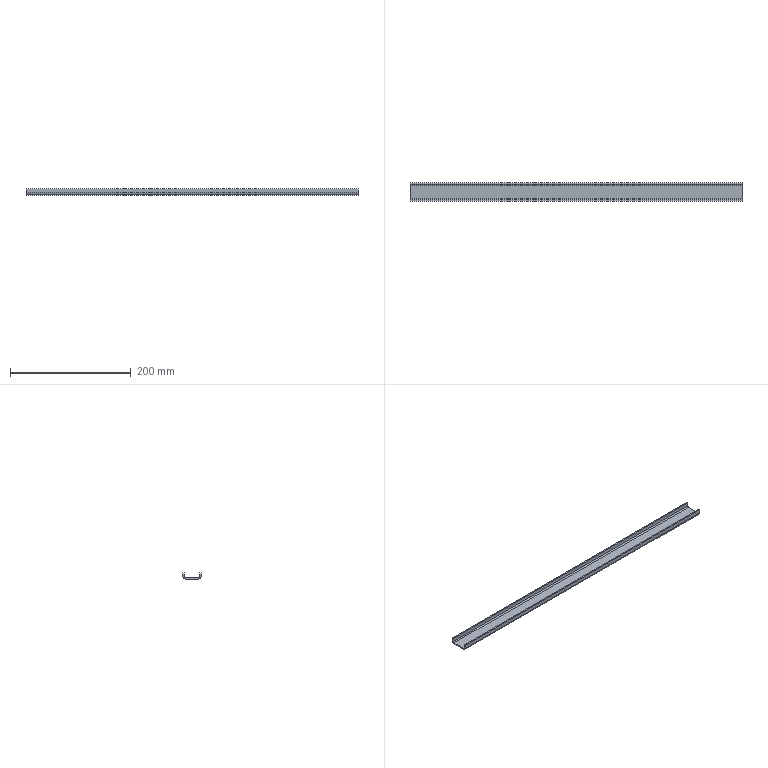Part | NX | features solid 2 | 1 solid | 14 faces | box 550 x 30 x 10 mm | volume 47767 mm3 | plane 10 | cylinder 4 | commonest cylinder face diameters 4 x2 8 x2
STEP:
#1=CARTESIAN_POINT('',(1955.,-1075.,1448.8));
#2=VERTEX_POINT('',#1);
#3=CARTESIAN_POINT('',(1955.,-1075.,1454.8));
#4=VERTEX_POINT('',#3);
#5=CARTESIAN_POINT('',(1955.,-1075.,1444.8));
#6=DIRECTION('',(0.,0.,1.));
#7=VECTOR('',#6,1000.);
#8=LINE('',#5,#7);
#9=EDGE_CURVE('',#2,#4,#8,.T.);
#10=ORIENTED_EDGE('',*,*,#9,.T.);
#11=CARTESIAN_POINT('',(1405.,-1075.,1454.8));
#12=VERTEX_POINT('',#11);
#13=CARTESIAN_POINT('',(1405.,-1075.,1454.8));
#14=DIRECTION('',(1.,0.,0.));
#15=VECTOR('',#14,1000.);
#16=LINE('',#13,#15);
#17=EDGE_CURVE('',#12,#4,#16,.T.);
#18=ORIENTED_EDGE('',*,*,#17,.F.);
#19=CARTESIAN_POINT('',(1405.,-1075.,1448.8));
#20=VERTEX_POINT('',#19);
#21=CARTESIAN_POINT('',(1405.,-1075.,1444.8));
#22=DIRECTION('',(0.,0.,1.));
#23=VECTOR('',#22,1000.);
#24=LINE('',#21,#23);
#25=EDGE_CURVE('',#20,#12,#24,.T.);
#26=ORIENTED_EDGE('',*,*,#25,.F.);
#27=CARTESIAN_POINT('',(1405.,-1075.,1448.8));
#28=DIRECTION('',(1.,0.,0.));
#29=VECTOR('',#28,1000.);
#30=LINE('',#27,#29);
#31=EDGE_CURVE('',#20,#2,#30,.T.);
#32=ORIENTED_EDGE('',*,*,#31,.T.);
#33=EDGE_LOOP('',(#10,#18,#26,#32));
#34=FACE_BOUND('',#33,.T.);
#35=CARTESIAN_POINT('',(1405.,-1075.,1444.8));
#36=DIRECTION('',(0.,1.,0.));
#37=DIRECTION('',(0.,0.,-1.));
#38=AXIS2_PLACEMENT_3D('',#35,#36,#37);
#39=PLANE('',#38);
#40=ADVANCED_FACE('',(#34),#39,.F.);
#41=CARTESIAN_POINT('',(1955.,-1077.,1446.8));
#42=VERTEX_POINT('',#41);
#43=CARTESIAN_POINT('',(1955.,-1077.,1448.8));
#44=DIRECTION('',(1.,0.,0.));
#45=DIRECTION('',(0.,0.,-1.));
#46=AXIS2_PLACEMENT_3D('',#43,#44,#45);
#47=CIRCLE('',#46,2.);
#48=EDGE_CURVE('',#42,#2,#47,.T.);
#49=ORIENTED_EDGE('',*,*,#48,.T.);
#50=ORIENTED_EDGE('',*,*,#31,.F.);
#51=CARTESIAN_POINT('',(1405.,-1077.,1446.8));
#52=VERTEX_POINT('',#51);
#53=CARTESIAN_POINT('',(1405.,-1077.,1448.8));
#54=DIRECTION('',(1.,0.,0.));
#55=DIRECTION('',(0.,0.,-1.));
#56=AXIS2_PLACEMENT_3D('',#53,#54,#55);
#57=CIRCLE('',#56,2.);
#58=EDGE_CURVE('',#52,#20,#57,.T.);
#59=ORIENTED_EDGE('',*,*,#58,.F.);
#60=CARTESIAN_POINT('',(1405.,-1077.,1446.8));
#61=DIRECTION('',(1.,0.,0.));
#62=VECTOR('',#61,1000.);
#63=LINE('',#60,#62);
#64=EDGE_CURVE('',#52,#42,#63,.T.);
#65=ORIENTED_EDGE('',*,*,#64,.T.);
#66=EDGE_LOOP('',(#49,#50,#59,#65));
#67=FACE_BOUND('',#66,.T.);
#68=CARTESIAN_POINT('',(1405.,-1077.,1448.8));
#69=DIRECTION('',(1.,0.,0.));
#70=DIRECTION('',(0.,0.,-1.));
#71=AXIS2_PLACEMENT_3D('',#68,#69,#70);
#72=CYLINDRICAL_SURFACE('',#71,2.);
#73=ADVANCED_FACE('',(#67),#72,.F.);
#74=CARTESIAN_POINT('',(1955.,-1099.,1446.8));
#75=VERTEX_POINT('',#74);
#76=CARTESIAN_POINT('',(1955.,-1103.,1446.8));
#77=DIRECTION('',(0.,1.,0.));
#78=VECTOR('',#77,1000.);
#79=LINE('',#76,#78);
#80=EDGE_CURVE('',#75,#42,#79,.T.);
#81=ORIENTED_EDGE('',*,*,#80,.T.);
#82=ORIENTED_EDGE('',*,*,#64,.F.);
#83=CARTESIAN_POINT('',(1405.,-1099.,1446.8));
#84=VERTEX_POINT('',#83);
#85=CARTESIAN_POINT('',(1405.,-1103.,1446.8));
#86=DIRECTION('',(0.,1.,0.));
#87=VECTOR('',#86,1000.);
#88=LINE('',#85,#87);
#89=EDGE_CURVE('',#84,#52,#88,.T.);
#90=ORIENTED_EDGE('',*,*,#89,.F.);
#91=CARTESIAN_POINT('',(1405.,-1099.,1446.8));
#92=DIRECTION('',(1.,0.,0.));
#93=VECTOR('',#92,1000.);
#94=LINE('',#91,#93);
#95=EDGE_CURVE('',#84,#75,#94,.T.);
#96=ORIENTED_EDGE('',*,*,#95,.T.);
#97=EDGE_LOOP('',(#81,#82,#90,#96));
#98=FACE_BOUND('',#97,.T.);
#99=CARTESIAN_POINT('',(1405.,-1103.,1446.8));
#100=DIRECTION('',(0.,0.,-1.));
#101=DIRECTION('',(0.,-1.,0.));
#102=AXIS2_PLACEMENT_3D('',#99,#100,#101);
#103=PLANE('',#102);
#104=ADVANCED_FACE('',(#98),#103,.F.);
#105=CARTESIAN_POINT('',(1955.,-1101.,1448.8));
#106=VERTEX_POINT('',#105);
#107=CARTESIAN_POINT('',(1955.,-1099.,1448.8));
#108=DIRECTION('',(1.,0.,0.));
#109=DIRECTION('',(0.,0.,-1.));
#110=AXIS2_PLACEMENT_3D('',#107,#108,#109);
#111=CIRCLE('',#110,2.);
#112=EDGE_CURVE('',#106,#75,#111,.T.);
#113=ORIENTED_EDGE('',*,*,#112,.T.);
#114=ORIENTED_EDGE('',*,*,#95,.F.);
#115=CARTESIAN_POINT('',(1405.,-1101.,1448.8));
#116=VERTEX_POINT('',#115);
#117=CARTESIAN_POINT('',(1405.,-1099.,1448.8));
#118=DIRECTION('',(1.,0.,0.));
#119=DIRECTION('',(0.,0.,-1.));
#120=AXIS2_PLACEMENT_3D('',#117,#118,#119);
#121=CIRCLE('',#120,2.);
#122=EDGE_CURVE('',#116,#84,#121,.T.);
#123=ORIENTED_EDGE('',*,*,#122,.F.);
#124=CARTESIAN_POINT('',(1405.,-1101.,1448.8));
#125=DIRECTION('',(1.,0.,0.));
#126=VECTOR('',#125,1000.);
#127=LINE('',#124,#126);
#128=EDGE_CURVE('',#116,#106,#127,.T.);
#129=ORIENTED_EDGE('',*,*,#128,.T.);
#130=EDGE_LOOP('',(#113,#114,#123,#129));
#131=FACE_BOUND('',#130,.T.);
#132=CARTESIAN_POINT('',(1405.,-1099.,1448.8));
#133=DIRECTION('',(1.,0.,0.));
#134=DIRECTION('',(0.,0.,-1.));
#135=AXIS2_PLACEMENT_3D('',#132,#133,#134);
#136=CYLINDRICAL_SURFACE('',#135,2.);
#137=ADVANCED_FACE('',(#131),#136,.F.);
#138=CARTESIAN_POINT('',(1955.,-1101.,1454.8));
#139=VERTEX_POINT('',#138);
#140=CARTESIAN_POINT('',(1955.,-1101.,1454.8));
#141=DIRECTION('',(0.,0.,-1.));
#142=VECTOR('',#141,1000.);
#143=LINE('',#140,#142);
#144=EDGE_CURVE('',#139,#106,#143,.T.);
#145=ORIENTED_EDGE('',*,*,#144,.T.);
#146=ORIENTED_EDGE('',*,*,#128,.F.);
#147=CARTESIAN_POINT('',(1405.,-1101.,1454.8));
#148=VERTEX_POINT('',#147);
#149=CARTESIAN_POINT('',(1405.,-1101.,1454.8));
#150=DIRECTION('',(0.,0.,-1.));
#151=VECTOR('',#150,1000.);
#152=LINE('',#149,#151);
#153=EDGE_CURVE('',#148,#116,#152,.T.);
#154=ORIENTED_EDGE('',*,*,#153,.F.);
#155=CARTESIAN_POINT('',(1405.,-1101.,1454.8));
#156=DIRECTION('',(1.,0.,0.));
#157=VECTOR('',#156,1000.);
#158=LINE('',#155,#157);
#159=EDGE_CURVE('',#148,#139,#158,.T.);
#160=ORIENTED_EDGE('',*,*,#159,.T.);
#161=EDGE_LOOP('',(#145,#146,#154,#160));
#162=FACE_BOUND('',#161,.T.);
#163=CARTESIAN_POINT('',(1405.,-1101.,1454.8));
#164=DIRECTION('',(0.,-1.,0.));
#165=DIRECTION('',(-1.,0.,0.));
#166=AXIS2_PLACEMENT_3D('',#163,#164,#165);
#167=PLANE('',#166);
#168=ADVANCED_FACE('',(#162),#167,.F.);
#169=CARTESIAN_POINT('',(1955.,-1073.,1448.8));
#170=VERTEX_POINT('',#169);
#171=CARTESIAN_POINT('',(1955.,-1073.,1454.8));
#172=VERTEX_POINT('',#171);
#173=CARTESIAN_POINT('',(1955.,-1073.,1444.8));
#174=DIRECTION('',(0.,0.,1.));
#175=VECTOR('',#174,1000.);
#176=LINE('',#173,#175);
#177=EDGE_CURVE('',#170,#172,#176,.T.);
#178=ORIENTED_EDGE('',*,*,#177,.F.);
#179=CARTESIAN_POINT('',(1405.,-1073.,1448.8));
#180=VERTEX_POINT('',#179);
#181=CARTESIAN_POINT('',(1405.,-1073.,1448.8));
#182=DIRECTION('',(1.,0.,0.));
#183=VECTOR('',#182,1000.);
#184=LINE('',#181,#183);
#185=EDGE_CURVE('',#180,#170,#184,.T.);
#186=ORIENTED_EDGE('',*,*,#185,.F.);
#187=CARTESIAN_POINT('',(1405.,-1073.,1454.8));
#188=VERTEX_POINT('',#187);
#189=CARTESIAN_POINT('',(1405.,-1073.,1444.8));
#190=DIRECTION('',(0.,0.,1.));
#191=VECTOR('',#190,1000.);
#192=LINE('',#189,#191);
#193=EDGE_CURVE('',#180,#188,#192,.T.);
#194=ORIENTED_EDGE('',*,*,#193,.T.);
#195=CARTESIAN_POINT('',(1405.,-1073.,1454.8));
#196=DIRECTION('',(1.,0.,0.));
#197=VECTOR('',#196,1000.);
#198=LINE('',#195,#197);
#199=EDGE_CURVE('',#188,#172,#198,.T.);
#200=ORIENTED_EDGE('',*,*,#199,.T.);
#201=EDGE_LOOP('',(#178,#186,#194,#200));
#202=FACE_BOUND('',#201,.T.);
#203=CARTESIAN_POINT('',(1405.,-1073.,1444.8));
#204=DIRECTION('',(0.,1.,0.));
#205=DIRECTION('',(0.,0.,-1.));
#206=AXIS2_PLACEMENT_3D('',#203,#204,#205);
#207=PLANE('',#206);
#208=ADVANCED_FACE('',(#202),#207,.T.);
#209=CARTESIAN_POINT('',(1955.,-1077.,1444.8));
#210=VERTEX_POINT('',#209);
#211=CARTESIAN_POINT('',(1955.,-1077.,1448.8));
#212=DIRECTION('',(1.,0.,0.));
#213=DIRECTION('',(0.,0.,1.));
#214=AXIS2_PLACEMENT_3D('',#211,#212,#213);
#215=CIRCLE('',#214,4.);
#216=EDGE_CURVE('',#210,#170,#215,.T.);
#217=ORIENTED_EDGE('',*,*,#216,.F.);
#218=CARTESIAN_POINT('',(1405.,-1077.,1444.8));
#219=VERTEX_POINT('',#218);
#220=CARTESIAN_POINT('',(1405.,-1077.,1444.8));
#221=DIRECTION('',(1.,0.,0.));
#222=VECTOR('',#221,1000.);
#223=LINE('',#220,#222);
#224=EDGE_CURVE('',#219,#210,#223,.T.);
#225=ORIENTED_EDGE('',*,*,#224,.F.);
#226=CARTESIAN_POINT('',(1405.,-1077.,1448.8));
#227=DIRECTION('',(1.,0.,0.));
#228=DIRECTION('',(0.,0.,1.));
#229=AXIS2_PLACEMENT_3D('',#226,#227,#228);
#230=CIRCLE('',#229,4.);
#231=EDGE_CURVE('',#219,#180,#230,.T.);
#232=ORIENTED_EDGE('',*,*,#231,.T.);
#233=ORIENTED_EDGE('',*,*,#185,.T.);
#234=EDGE_LOOP('',(#217,#225,#232,#233));
#235=FACE_BOUND('',#234,.T.);
#236=CARTESIAN_POINT('',(1405.,-1077.,1448.8));
#237=DIRECTION('',(1.,0.,0.));
#238=DIRECTION('',(0.,0.,-1.));
#239=AXIS2_PLACEMENT_3D('',#236,#237,#238);
#240=CYLINDRICAL_SURFACE('',#239,4.);
#241=ADVANCED_FACE('',(#235),#240,.T.);
#242=CARTESIAN_POINT('',(1955.,-1099.,1444.8));
#243=VERTEX_POINT('',#242);
#244=CARTESIAN_POINT('',(1955.,-1103.,1444.8));
#245=DIRECTION('',(0.,1.,0.));
#246=VECTOR('',#245,1000.);
#247=LINE('',#244,#246);
#248=EDGE_CURVE('',#243,#210,#247,.T.);
#249=ORIENTED_EDGE('',*,*,#248,.F.);
#250=CARTESIAN_POINT('',(1405.,-1099.,1444.8));
#251=VERTEX_POINT('',#250);
#252=CARTESIAN_POINT('',(1405.,-1099.,1444.8));
#253=DIRECTION('',(1.,0.,0.));
#254=VECTOR('',#253,1000.);
#255=LINE('',#252,#254);
#256=EDGE_CURVE('',#251,#243,#255,.T.);
#257=ORIENTED_EDGE('',*,*,#256,.F.);
#258=CARTESIAN_POINT('',(1405.,-1103.,1444.8));
#259=DIRECTION('',(0.,1.,0.));
#260=VECTOR('',#259,1000.);
#261=LINE('',#258,#260);
#262=EDGE_CURVE('',#251,#219,#261,.T.);
#263=ORIENTED_EDGE('',*,*,#262,.T.);
#264=ORIENTED_EDGE('',*,*,#224,.T.);
#265=EDGE_LOOP('',(#249,#257,#263,#264));
#266=FACE_BOUND('',#265,.T.);
#267=CARTESIAN_POINT('',(1405.,-1103.,1444.8));
#268=DIRECTION('',(0.,0.,-1.));
#269=DIRECTION('',(0.,-1.,0.));
#270=AXIS2_PLACEMENT_3D('',#267,#268,#269);
#271=PLANE('',#270);
#272=ADVANCED_FACE('',(#266),#271,.T.);
#273=CARTESIAN_POINT('',(1955.,-1103.,1448.8));
#274=VERTEX_POINT('',#273);
#275=CARTESIAN_POINT('',(1955.,-1099.,1448.8));
#276=DIRECTION('',(1.,0.,0.));
#277=DIRECTION('',(0.,0.,1.));
#278=AXIS2_PLACEMENT_3D('',#275,#276,#277);
#279=CIRCLE('',#278,4.);
#280=EDGE_CURVE('',#274,#243,#279,.T.);
#281=ORIENTED_EDGE('',*,*,#280,.F.);
#282=CARTESIAN_POINT('',(1405.,-1103.,1448.8));
#283=VERTEX_POINT('',#282);
#284=CARTESIAN_POINT('',(1405.,-1103.,1448.8));
#285=DIRECTION('',(1.,0.,0.));
#286=VECTOR('',#285,1000.);
#287=LINE('',#284,#286);
#288=EDGE_CURVE('',#283,#274,#287,.T.);
#289=ORIENTED_EDGE('',*,*,#288,.F.);
#290=CARTESIAN_POINT('',(1405.,-1099.,1448.8));
#291=DIRECTION('',(1.,0.,0.));
#292=DIRECTION('',(0.,0.,1.));
#293=AXIS2_PLACEMENT_3D('',#290,#291,#292);
#294=CIRCLE('',#293,4.);
#295=EDGE_CURVE('',#283,#251,#294,.T.);
#296=ORIENTED_EDGE('',*,*,#295,.T.);
#297=ORIENTED_EDGE('',*,*,#256,.T.);
#298=EDGE_LOOP('',(#281,#289,#296,#297));
#299=FACE_BOUND('',#298,.T.);
#300=CARTESIAN_POINT('',(1405.,-1099.,1448.8));
#301=DIRECTION('',(1.,0.,0.));
#302=DIRECTION('',(0.,0.,-1.));
#303=AXIS2_PLACEMENT_3D('',#300,#301,#302);
#304=CYLINDRICAL_SURFACE('',#303,4.);
#305=ADVANCED_FACE('',(#299),#304,.T.);
#306=CARTESIAN_POINT('',(1955.,-1103.,1454.8));
#307=VERTEX_POINT('',#306);
#308=CARTESIAN_POINT('',(1955.,-1103.,1454.8));
#309=DIRECTION('',(0.,0.,-1.));
#310=VECTOR('',#309,1000.);
#311=LINE('',#308,#310);
#312=EDGE_CURVE('',#307,#274,#311,.T.);
#313=ORIENTED_EDGE('',*,*,#312,.F.);
#314=CARTESIAN_POINT('',(1405.,-1103.,1454.8));
#315=VERTEX_POINT('',#314);
#316=CARTESIAN_POINT('',(1405.,-1103.,1454.8));
#317=DIRECTION('',(1.,0.,0.));
#318=VECTOR('',#317,1000.);
#319=LINE('',#316,#318);
#320=EDGE_CURVE('',#315,#307,#319,.T.);
#321=ORIENTED_EDGE('',*,*,#320,.F.);
#322=CARTESIAN_POINT('',(1405.,-1103.,1454.8));
#323=DIRECTION('',(0.,0.,-1.));
#324=VECTOR('',#323,1000.);
#325=LINE('',#322,#324);
#326=EDGE_CURVE('',#315,#283,#325,.T.);
#327=ORIENTED_EDGE('',*,*,#326,.T.);
#328=ORIENTED_EDGE('',*,*,#288,.T.);
#329=EDGE_LOOP('',(#313,#321,#327,#328));
#330=FACE_BOUND('',#329,.T.);
#331=CARTESIAN_POINT('',(1405.,-1103.,1454.8));
#332=DIRECTION('',(0.,-1.,0.));
#333=DIRECTION('',(-1.,0.,0.));
#334=AXIS2_PLACEMENT_3D('',#331,#332,#333);
#335=PLANE('',#334);
#336=ADVANCED_FACE('',(#330),#335,.T.);
#337=ORIENTED_EDGE('',*,*,#159,.F.);
#338=CARTESIAN_POINT('',(1405.,-1103.,1454.8));
#339=DIRECTION('',(0.,-1.,0.));
#340=VECTOR('',#339,1000.);
#341=LINE('',#338,#340);
#342=EDGE_CURVE('',#148,#315,#341,.T.);
#343=ORIENTED_EDGE('',*,*,#342,.T.);
#344=ORIENTED_EDGE('',*,*,#320,.T.);
#345=CARTESIAN_POINT('',(1955.,-1103.,1454.8));
#346=DIRECTION('',(0.,-1.,0.));
#347=VECTOR('',#346,1000.);
#348=LINE('',#345,#347);
#349=EDGE_CURVE('',#139,#307,#348,.T.);
#350=ORIENTED_EDGE('',*,*,#349,.F.);
#351=EDGE_LOOP('',(#337,#343,#344,#350));
#352=FACE_BOUND('',#351,.T.);
#353=CARTESIAN_POINT('',(1405.,-1103.,1454.8));
#354=DIRECTION('',(0.,0.,-1.));
#355=DIRECTION('',(0.,-1.,0.));
#356=AXIS2_PLACEMENT_3D('',#353,#354,#355);
#357=PLANE('',#356);
#358=ADVANCED_FACE('',(#352),#357,.F.);
#359=ORIENTED_EDGE('',*,*,#312,.T.);
#360=ORIENTED_EDGE('',*,*,#280,.T.);
#361=ORIENTED_EDGE('',*,*,#248,.T.);
#362=ORIENTED_EDGE('',*,*,#216,.T.);
#363=ORIENTED_EDGE('',*,*,#177,.T.);
#364=CARTESIAN_POINT('',(1955.,-1073.,1454.8));
#365=DIRECTION('',(0.,1.,0.));
#366=VECTOR('',#365,1000.);
#367=LINE('',#364,#366);
#368=EDGE_CURVE('',#4,#172,#367,.T.);
#369=ORIENTED_EDGE('',*,*,#368,.F.);
#370=ORIENTED_EDGE('',*,*,#9,.F.);
#371=ORIENTED_EDGE('',*,*,#48,.F.);
#372=ORIENTED_EDGE('',*,*,#80,.F.);
#373=ORIENTED_EDGE('',*,*,#112,.F.);
#374=ORIENTED_EDGE('',*,*,#144,.F.);
#375=ORIENTED_EDGE('',*,*,#349,.T.);
#376=EDGE_LOOP('',(#359,#360,#361,#362,#363,#369,#370,#371,#372,#373,#374,#375));
#377=FACE_BOUND('',#376,.T.);
#378=CARTESIAN_POINT('',(1955.,-1103.,1454.8));
#379=DIRECTION('',(-1.,0.,0.));
#380=DIRECTION('',(0.,0.,1.));
#381=AXIS2_PLACEMENT_3D('',#378,#379,#380);
#382=PLANE('',#381);
#383=ADVANCED_FACE('',(#377),#382,.F.);
#384=CARTESIAN_POINT('',(1405.,-1073.,1454.8));
#385=DIRECTION('',(0.,1.,0.));
#386=VECTOR('',#385,1000.);
#387=LINE('',#384,#386);
#388=EDGE_CURVE('',#12,#188,#387,.T.);
#389=ORIENTED_EDGE('',*,*,#388,.F.);
#390=ORIENTED_EDGE('',*,*,#17,.T.);
#391=ORIENTED_EDGE('',*,*,#368,.T.);
#392=ORIENTED_EDGE('',*,*,#199,.F.);
#393=EDGE_LOOP('',(#389,#390,#391,#392));
#394=FACE_BOUND('',#393,.T.);
#395=CARTESIAN_POINT('',(1405.,-1073.,1454.8));
#396=DIRECTION('',(0.,0.,1.));
#397=DIRECTION('',(1.,0.,0.));
#398=AXIS2_PLACEMENT_3D('',#395,#396,#397);
#399=PLANE('',#398);
#400=ADVANCED_FACE('',(#394),#399,.T.);
#401=ORIENTED_EDGE('',*,*,#193,.F.);
#402=ORIENTED_EDGE('',*,*,#231,.F.);
#403=ORIENTED_EDGE('',*,*,#262,.F.);
#404=ORIENTED_EDGE('',*,*,#295,.F.);
#405=ORIENTED_EDGE('',*,*,#326,.F.);
#406=ORIENTED_EDGE('',*,*,#342,.F.);
#407=ORIENTED_EDGE('',*,*,#153,.T.);
#408=ORIENTED_EDGE('',*,*,#122,.T.);
#409=ORIENTED_EDGE('',*,*,#89,.T.);
#410=ORIENTED_EDGE('',*,*,#58,.T.);
#411=ORIENTED_EDGE('',*,*,#25,.T.);
#412=ORIENTED_EDGE('',*,*,#388,.T.);
#413=EDGE_LOOP('',(#401,#402,#403,#404,#405,#406,#407,#408,#409,#410,#411,#412));
#414=FACE_BOUND('',#413,.T.);
#415=CARTESIAN_POINT('',(1405.,-1073.,1444.8));
#416=DIRECTION('',(-1.,0.,0.));
#417=DIRECTION('',(0.,0.,1.));
#418=AXIS2_PLACEMENT_3D('',#415,#416,#417);
#419=PLANE('',#418);
#420=ADVANCED_FACE('',(#414),#419,.T.);
#421=CLOSED_SHELL('',(#40,#73,#104,#137,#168,#208,#241,#272,#305,#336,#358,#383,#400,#420));
#422=MANIFOLD_SOLID_BREP('',#421);
#423=(LENGTH_UNIT()NAMED_UNIT(*)SI_UNIT(.MILLI.,.METRE.));
#424=UNCERTAINTY_MEASURE_WITH_UNIT(LENGTH_MEASURE(0.00001),#423,'','');
#425=(NAMED_UNIT(*)PLANE_ANGLE_UNIT()SI_UNIT($,.RADIAN.));
#426=(NAMED_UNIT(*)SI_UNIT($,.STERADIAN.)SOLID_ANGLE_UNIT());
#427=(GEOMETRIC_REPRESENTATION_CONTEXT(3)GLOBAL_UNCERTAINTY_ASSIGNED_CONTEXT((#424))GLOBAL_UNIT_ASSIGNED_CONTEXT((#423,#425,#426))REPRESENTATION_CONTEXT('',''));
#428=ADVANCED_BREP_SHAPE_REPRESENTATION('',(#422),#427);